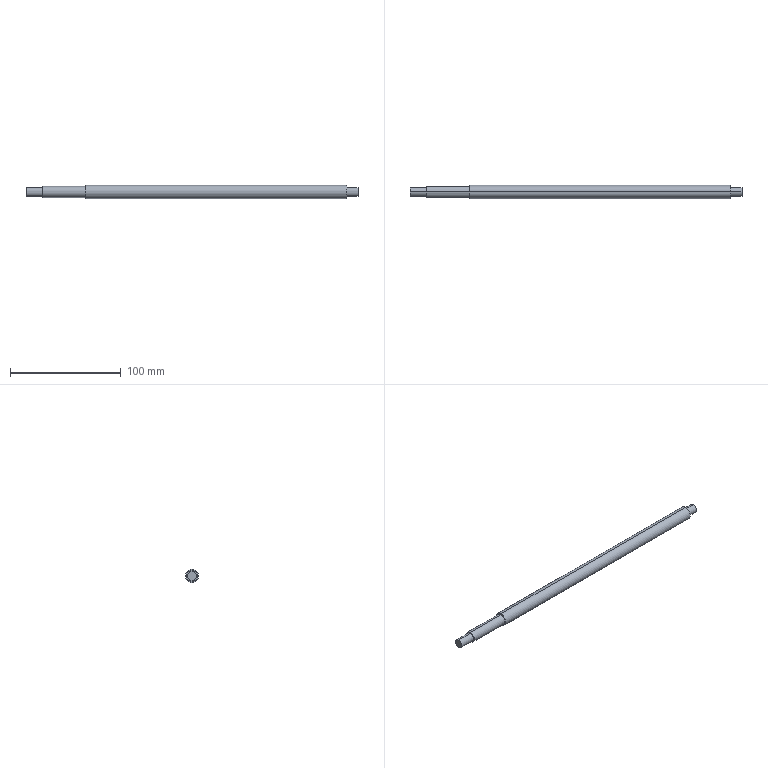Part | SolidWorks | features BaseBody 1 | 1 solid | 13 faces | box 300 x 12 x 12 mm | volume 31011 mm3 | cylinder 8 | plane 5 | commonest cylinder face diameters 8 x4 10 x2 12 x2
STEP:
#1=CARTESIAN_POINT('',(290.,0.,6.));
#2=VERTEX_POINT('',#1);
#3=CARTESIAN_POINT('',(290.,0.,-6.));
#4=VERTEX_POINT('',#3);
#5=CARTESIAN_POINT('',(290.,0.,0.));
#6=DIRECTION('',(-1.,0.,0.));
#7=DIRECTION('',(0.,0.,1.));
#8=AXIS2_PLACEMENT_3D('',#5,#6,#7);
#9=CIRCLE('',#8,6.);
#10=EDGE_CURVE('',#2,#4,#9,.T.);
#11=ORIENTED_EDGE('',*,*,#10,.T.);
#12=CARTESIAN_POINT('',(54.,0.,-6.));
#13=VERTEX_POINT('',#12);
#14=CARTESIAN_POINT('',(0.,0.,-6.));
#15=DIRECTION('',(-1.,0.,0.));
#16=VECTOR('',#15,1000.);
#17=LINE('',#14,#16);
#18=EDGE_CURVE('',#4,#13,#17,.T.);
#19=ORIENTED_EDGE('',*,*,#18,.T.);
#20=CARTESIAN_POINT('',(54.,0.,6.));
#21=VERTEX_POINT('',#20);
#22=CARTESIAN_POINT('',(54.,0.,0.));
#23=DIRECTION('',(1.,0.,0.));
#24=DIRECTION('',(0.,0.,1.));
#25=AXIS2_PLACEMENT_3D('',#22,#23,#24);
#26=CIRCLE('',#25,6.);
#27=EDGE_CURVE('',#13,#21,#26,.T.);
#28=ORIENTED_EDGE('',*,*,#27,.T.);
#29=CARTESIAN_POINT('',(0.,0.,6.));
#30=DIRECTION('',(-1.,0.,0.));
#31=VECTOR('',#30,1000.);
#32=LINE('',#29,#31);
#33=EDGE_CURVE('',#2,#21,#32,.T.);
#34=ORIENTED_EDGE('',*,*,#33,.F.);
#35=EDGE_LOOP('',(#11,#19,#28,#34));
#36=FACE_OUTER_BOUND('',#35,.T.);
#37=CARTESIAN_POINT('',(0.,0.,0.));
#38=DIRECTION('',(-1.,0.,0.));
#39=DIRECTION('',(0.,0.,1.));
#40=AXIS2_PLACEMENT_3D('',#37,#38,#39);
#41=CYLINDRICAL_SURFACE('',#40,6.);
#42=ADVANCED_FACE('',(#36),#41,.T.);
#43=CARTESIAN_POINT('',(54.,0.,5.));
#44=VERTEX_POINT('',#43);
#45=CARTESIAN_POINT('',(54.,0.,-5.));
#46=VERTEX_POINT('',#45);
#47=CARTESIAN_POINT('',(54.,0.,0.));
#48=DIRECTION('',(-1.,0.,0.));
#49=DIRECTION('',(0.,0.,1.));
#50=AXIS2_PLACEMENT_3D('',#47,#48,#49);
#51=CIRCLE('',#50,5.);
#52=EDGE_CURVE('',#44,#46,#51,.T.);
#53=ORIENTED_EDGE('',*,*,#52,.T.);
#54=CARTESIAN_POINT('',(15.,0.,-5.));
#55=VERTEX_POINT('',#54);
#56=CARTESIAN_POINT('',(0.,0.,-5.));
#57=DIRECTION('',(-1.,0.,0.));
#58=VECTOR('',#57,1000.);
#59=LINE('',#56,#58);
#60=EDGE_CURVE('',#46,#55,#59,.T.);
#61=ORIENTED_EDGE('',*,*,#60,.T.);
#62=CARTESIAN_POINT('',(15.,0.,5.));
#63=VERTEX_POINT('',#62);
#64=CARTESIAN_POINT('',(15.,0.,0.));
#65=DIRECTION('',(1.,0.,0.));
#66=DIRECTION('',(0.,0.,1.));
#67=AXIS2_PLACEMENT_3D('',#64,#65,#66);
#68=CIRCLE('',#67,5.);
#69=EDGE_CURVE('',#55,#63,#68,.T.);
#70=ORIENTED_EDGE('',*,*,#69,.T.);
#71=CARTESIAN_POINT('',(0.,0.,5.));
#72=DIRECTION('',(-1.,0.,0.));
#73=VECTOR('',#72,1000.);
#74=LINE('',#71,#73);
#75=EDGE_CURVE('',#44,#63,#74,.T.);
#76=ORIENTED_EDGE('',*,*,#75,.F.);
#77=EDGE_LOOP('',(#53,#61,#70,#76));
#78=FACE_OUTER_BOUND('',#77,.T.);
#79=CARTESIAN_POINT('',(0.,0.,0.));
#80=DIRECTION('',(-1.,0.,0.));
#81=DIRECTION('',(0.,0.,1.));
#82=AXIS2_PLACEMENT_3D('',#79,#80,#81);
#83=CYLINDRICAL_SURFACE('',#82,5.);
#84=ADVANCED_FACE('',(#78),#83,.T.);
#85=CARTESIAN_POINT('',(300.,0.,4.));
#86=VERTEX_POINT('',#85);
#87=CARTESIAN_POINT('',(300.,0.,-4.));
#88=VERTEX_POINT('',#87);
#89=CARTESIAN_POINT('',(300.,0.,0.));
#90=DIRECTION('',(-1.,0.,0.));
#91=DIRECTION('',(0.,0.,1.));
#92=AXIS2_PLACEMENT_3D('',#89,#90,#91);
#93=CIRCLE('',#92,4.);
#94=EDGE_CURVE('',#86,#88,#93,.T.);
#95=ORIENTED_EDGE('',*,*,#94,.T.);
#96=CARTESIAN_POINT('',(290.,0.,-4.));
#97=VERTEX_POINT('',#96);
#98=CARTESIAN_POINT('',(0.,0.,-4.));
#99=DIRECTION('',(-1.,0.,0.));
#100=VECTOR('',#99,1000.);
#101=LINE('',#98,#100);
#102=EDGE_CURVE('',#88,#97,#101,.T.);
#103=ORIENTED_EDGE('',*,*,#102,.T.);
#104=CARTESIAN_POINT('',(290.,0.,4.));
#105=VERTEX_POINT('',#104);
#106=CARTESIAN_POINT('',(290.,0.,0.));
#107=DIRECTION('',(1.,0.,0.));
#108=DIRECTION('',(0.,0.,1.));
#109=AXIS2_PLACEMENT_3D('',#106,#107,#108);
#110=CIRCLE('',#109,4.);
#111=EDGE_CURVE('',#97,#105,#110,.T.);
#112=ORIENTED_EDGE('',*,*,#111,.T.);
#113=CARTESIAN_POINT('',(0.,0.,4.));
#114=DIRECTION('',(-1.,0.,0.));
#115=VECTOR('',#114,1000.);
#116=LINE('',#113,#115);
#117=EDGE_CURVE('',#86,#105,#116,.T.);
#118=ORIENTED_EDGE('',*,*,#117,.F.);
#119=EDGE_LOOP('',(#95,#103,#112,#118));
#120=FACE_OUTER_BOUND('',#119,.T.);
#121=CARTESIAN_POINT('',(0.,0.,0.));
#122=DIRECTION('',(-1.,0.,0.));
#123=DIRECTION('',(0.,0.,1.));
#124=AXIS2_PLACEMENT_3D('',#121,#122,#123);
#125=CYLINDRICAL_SURFACE('',#124,4.);
#126=ADVANCED_FACE('',(#120),#125,.T.);
#127=CARTESIAN_POINT('',(15.,0.,4.));
#128=VERTEX_POINT('',#127);
#129=CARTESIAN_POINT('',(15.,0.,-4.));
#130=VERTEX_POINT('',#129);
#131=CARTESIAN_POINT('',(15.,0.,0.));
#132=DIRECTION('',(-1.,0.,0.));
#133=DIRECTION('',(0.,0.,1.));
#134=AXIS2_PLACEMENT_3D('',#131,#132,#133);
#135=CIRCLE('',#134,4.);
#136=EDGE_CURVE('',#128,#130,#135,.T.);
#137=ORIENTED_EDGE('',*,*,#136,.T.);
#138=CARTESIAN_POINT('',(0.,0.,-4.));
#139=VERTEX_POINT('',#138);
#140=CARTESIAN_POINT('',(0.,0.,-4.));
#141=DIRECTION('',(-1.,0.,0.));
#142=VECTOR('',#141,1000.);
#143=LINE('',#140,#142);
#144=EDGE_CURVE('',#130,#139,#143,.T.);
#145=ORIENTED_EDGE('',*,*,#144,.T.);
#146=CARTESIAN_POINT('',(0.,0.,4.));
#147=VERTEX_POINT('',#146);
#148=CARTESIAN_POINT('',(0.,0.,0.));
#149=DIRECTION('',(1.,0.,0.));
#150=DIRECTION('',(0.,0.,1.));
#151=AXIS2_PLACEMENT_3D('',#148,#149,#150);
#152=CIRCLE('',#151,4.);
#153=EDGE_CURVE('',#139,#147,#152,.T.);
#154=ORIENTED_EDGE('',*,*,#153,.T.);
#155=CARTESIAN_POINT('',(0.,0.,4.));
#156=DIRECTION('',(-1.,0.,0.));
#157=VECTOR('',#156,1000.);
#158=LINE('',#155,#157);
#159=EDGE_CURVE('',#128,#147,#158,.T.);
#160=ORIENTED_EDGE('',*,*,#159,.F.);
#161=EDGE_LOOP('',(#137,#145,#154,#160));
#162=FACE_OUTER_BOUND('',#161,.T.);
#163=CARTESIAN_POINT('',(0.,0.,0.));
#164=DIRECTION('',(-1.,0.,0.));
#165=DIRECTION('',(0.,0.,1.));
#166=AXIS2_PLACEMENT_3D('',#163,#164,#165);
#167=CYLINDRICAL_SURFACE('',#166,4.);
#168=ADVANCED_FACE('',(#162),#167,.T.);
#169=ORIENTED_EDGE('',*,*,#18,.F.);
#170=CARTESIAN_POINT('',(290.,0.,0.));
#171=DIRECTION('',(-1.,0.,0.));
#172=DIRECTION('',(0.,0.,1.));
#173=AXIS2_PLACEMENT_3D('',#170,#171,#172);
#174=CIRCLE('',#173,6.);
#175=EDGE_CURVE('',#4,#2,#174,.T.);
#176=ORIENTED_EDGE('',*,*,#175,.T.);
#177=ORIENTED_EDGE('',*,*,#33,.T.);
#178=CARTESIAN_POINT('',(54.,0.,0.));
#179=DIRECTION('',(1.,0.,0.));
#180=DIRECTION('',(0.,0.,1.));
#181=AXIS2_PLACEMENT_3D('',#178,#179,#180);
#182=CIRCLE('',#181,6.);
#183=EDGE_CURVE('',#21,#13,#182,.T.);
#184=ORIENTED_EDGE('',*,*,#183,.T.);
#185=EDGE_LOOP('',(#169,#176,#177,#184));
#186=FACE_OUTER_BOUND('',#185,.T.);
#187=CARTESIAN_POINT('',(0.,0.,0.));
#188=DIRECTION('',(-1.,0.,0.));
#189=DIRECTION('',(0.,0.,1.));
#190=AXIS2_PLACEMENT_3D('',#187,#188,#189);
#191=CYLINDRICAL_SURFACE('',#190,6.);
#192=ADVANCED_FACE('',(#186),#191,.T.);
#193=ORIENTED_EDGE('',*,*,#183,.F.);
#194=ORIENTED_EDGE('',*,*,#27,.F.);
#195=EDGE_LOOP('',(#193,#194));
#196=FACE_OUTER_BOUND('',#195,.T.);
#197=ORIENTED_EDGE('',*,*,#52,.F.);
#198=CARTESIAN_POINT('',(54.,0.,0.));
#199=DIRECTION('',(-1.,0.,0.));
#200=DIRECTION('',(0.,0.,1.));
#201=AXIS2_PLACEMENT_3D('',#198,#199,#200);
#202=CIRCLE('',#201,5.);
#203=EDGE_CURVE('',#46,#44,#202,.T.);
#204=ORIENTED_EDGE('',*,*,#203,.F.);
#205=EDGE_LOOP('',(#197,#204));
#206=FACE_BOUND('',#205,.T.);
#207=CARTESIAN_POINT('',(54.,5.,0.));
#208=DIRECTION('',(1.,0.,0.));
#209=DIRECTION('',(0.,0.,-1.));
#210=AXIS2_PLACEMENT_3D('',#207,#208,#209);
#211=PLANE('',#210);
#212=ADVANCED_FACE('',(#196,#206),#211,.F.);
#213=CARTESIAN_POINT('',(290.,0.,0.));
#214=DIRECTION('',(1.,0.,0.));
#215=DIRECTION('',(0.,0.,1.));
#216=AXIS2_PLACEMENT_3D('',#213,#214,#215);
#217=CIRCLE('',#216,4.);
#218=EDGE_CURVE('',#105,#97,#217,.T.);
#219=ORIENTED_EDGE('',*,*,#218,.F.);
#220=ORIENTED_EDGE('',*,*,#111,.F.);
#221=EDGE_LOOP('',(#219,#220));
#222=FACE_BOUND('',#221,.T.);
#223=ORIENTED_EDGE('',*,*,#10,.F.);
#224=ORIENTED_EDGE('',*,*,#175,.F.);
#225=EDGE_LOOP('',(#223,#224));
#226=FACE_OUTER_BOUND('',#225,.T.);
#227=CARTESIAN_POINT('',(290.,6.,0.));
#228=DIRECTION('',(-1.,0.,0.));
#229=DIRECTION('',(0.,0.,1.));
#230=AXIS2_PLACEMENT_3D('',#227,#228,#229);
#231=PLANE('',#230);
#232=ADVANCED_FACE('',(#222,#226),#231,.F.);
#233=ORIENTED_EDGE('',*,*,#60,.F.);
#234=ORIENTED_EDGE('',*,*,#203,.T.);
#235=ORIENTED_EDGE('',*,*,#75,.T.);
#236=CARTESIAN_POINT('',(15.,0.,0.));
#237=DIRECTION('',(1.,0.,0.));
#238=DIRECTION('',(0.,0.,1.));
#239=AXIS2_PLACEMENT_3D('',#236,#237,#238);
#240=CIRCLE('',#239,5.);
#241=EDGE_CURVE('',#63,#55,#240,.T.);
#242=ORIENTED_EDGE('',*,*,#241,.T.);
#243=EDGE_LOOP('',(#233,#234,#235,#242));
#244=FACE_OUTER_BOUND('',#243,.T.);
#245=CARTESIAN_POINT('',(0.,0.,0.));
#246=DIRECTION('',(-1.,0.,0.));
#247=DIRECTION('',(0.,0.,1.));
#248=AXIS2_PLACEMENT_3D('',#245,#246,#247);
#249=CYLINDRICAL_SURFACE('',#248,5.);
#250=ADVANCED_FACE('',(#244),#249,.T.);
#251=ORIENTED_EDGE('',*,*,#102,.F.);
#252=CARTESIAN_POINT('',(300.,0.,0.));
#253=DIRECTION('',(-1.,0.,0.));
#254=DIRECTION('',(0.,0.,1.));
#255=AXIS2_PLACEMENT_3D('',#252,#253,#254);
#256=CIRCLE('',#255,4.);
#257=EDGE_CURVE('',#88,#86,#256,.T.);
#258=ORIENTED_EDGE('',*,*,#257,.T.);
#259=ORIENTED_EDGE('',*,*,#117,.T.);
#260=ORIENTED_EDGE('',*,*,#218,.T.);
#261=EDGE_LOOP('',(#251,#258,#259,#260));
#262=FACE_OUTER_BOUND('',#261,.T.);
#263=CARTESIAN_POINT('',(0.,0.,0.));
#264=DIRECTION('',(-1.,0.,0.));
#265=DIRECTION('',(0.,0.,1.));
#266=AXIS2_PLACEMENT_3D('',#263,#264,#265);
#267=CYLINDRICAL_SURFACE('',#266,4.);
#268=ADVANCED_FACE('',(#262),#267,.T.);
#269=ORIENTED_EDGE('',*,*,#241,.F.);
#270=ORIENTED_EDGE('',*,*,#69,.F.);
#271=EDGE_LOOP('',(#269,#270));
#272=FACE_OUTER_BOUND('',#271,.T.);
#273=ORIENTED_EDGE('',*,*,#136,.F.);
#274=CARTESIAN_POINT('',(15.,0.,0.));
#275=DIRECTION('',(-1.,0.,0.));
#276=DIRECTION('',(0.,0.,1.));
#277=AXIS2_PLACEMENT_3D('',#274,#275,#276);
#278=CIRCLE('',#277,4.);
#279=EDGE_CURVE('',#130,#128,#278,.T.);
#280=ORIENTED_EDGE('',*,*,#279,.F.);
#281=EDGE_LOOP('',(#273,#280));
#282=FACE_BOUND('',#281,.T.);
#283=CARTESIAN_POINT('',(15.,4.,0.));
#284=DIRECTION('',(1.,0.,0.));
#285=DIRECTION('',(0.,0.,-1.));
#286=AXIS2_PLACEMENT_3D('',#283,#284,#285);
#287=PLANE('',#286);
#288=ADVANCED_FACE('',(#272,#282),#287,.F.);
#289=ORIENTED_EDGE('',*,*,#94,.F.);
#290=ORIENTED_EDGE('',*,*,#257,.F.);
#291=EDGE_LOOP('',(#289,#290));
#292=FACE_OUTER_BOUND('',#291,.T.);
#293=CARTESIAN_POINT('',(300.,4.,0.));
#294=DIRECTION('',(-1.,0.,0.));
#295=DIRECTION('',(0.,0.,1.));
#296=AXIS2_PLACEMENT_3D('',#293,#294,#295);
#297=PLANE('',#296);
#298=ADVANCED_FACE('',(#292),#297,.F.);
#299=ORIENTED_EDGE('',*,*,#144,.F.);
#300=ORIENTED_EDGE('',*,*,#279,.T.);
#301=ORIENTED_EDGE('',*,*,#159,.T.);
#302=CARTESIAN_POINT('',(0.,0.,0.));
#303=DIRECTION('',(1.,0.,0.));
#304=DIRECTION('',(0.,0.,1.));
#305=AXIS2_PLACEMENT_3D('',#302,#303,#304);
#306=CIRCLE('',#305,4.);
#307=EDGE_CURVE('',#147,#139,#306,.T.);
#308=ORIENTED_EDGE('',*,*,#307,.T.);
#309=EDGE_LOOP('',(#299,#300,#301,#308));
#310=FACE_OUTER_BOUND('',#309,.T.);
#311=CARTESIAN_POINT('',(0.,0.,0.));
#312=DIRECTION('',(-1.,0.,0.));
#313=DIRECTION('',(0.,0.,1.));
#314=AXIS2_PLACEMENT_3D('',#311,#312,#313);
#315=CYLINDRICAL_SURFACE('',#314,4.);
#316=ADVANCED_FACE('',(#310),#315,.T.);
#317=ORIENTED_EDGE('',*,*,#307,.F.);
#318=ORIENTED_EDGE('',*,*,#153,.F.);
#319=EDGE_LOOP('',(#317,#318));
#320=FACE_OUTER_BOUND('',#319,.T.);
#321=CARTESIAN_POINT('',(0.,0.,0.));
#322=DIRECTION('',(1.,0.,0.));
#323=DIRECTION('',(0.,0.,-1.));
#324=AXIS2_PLACEMENT_3D('',#321,#322,#323);
#325=PLANE('',#324);
#326=ADVANCED_FACE('',(#320),#325,.F.);
#327=CLOSED_SHELL('',(#42,#84,#126,#168,#192,#212,#232,#250,#268,#288,#298,#316,#326));
#328=MANIFOLD_SOLID_BREP('',#327);
#329=CARTESIAN_POINT('',(0.,0.,0.));
#330=DIRECTION('',(0.,0.,1.));
#331=DIRECTION('',(1.,0.,0.));
#332=AXIS2_PLACEMENT_3D('',#329,#330,#331);
#333=(LENGTH_UNIT()NAMED_UNIT(*)SI_UNIT(.MILLI.,.METRE.));
#334=UNCERTAINTY_MEASURE_WITH_UNIT(LENGTH_MEASURE(0.00001),#333,'','');
#335=(NAMED_UNIT(*)PLANE_ANGLE_UNIT()SI_UNIT($,.RADIAN.));
#336=(NAMED_UNIT(*)SI_UNIT($,.STERADIAN.)SOLID_ANGLE_UNIT());
#337=(GEOMETRIC_REPRESENTATION_CONTEXT(3)GLOBAL_UNCERTAINTY_ASSIGNED_CONTEXT((#334))GLOBAL_UNIT_ASSIGNED_CONTEXT((#333,#335,#336))REPRESENTATION_CONTEXT('',''));
#338=ADVANCED_BREP_SHAPE_REPRESENTATION('',(#328,#332),#337);